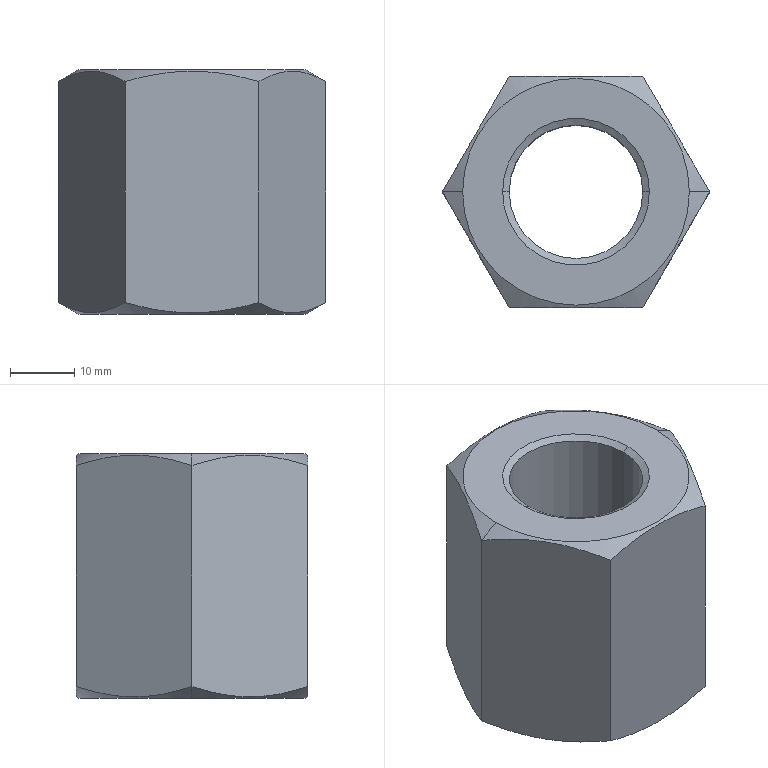Part | SolidWorks | features RevCut 2, Chamfer 1, Extrusion 1, LPattern 1 | 1 solid | 18 faces | box 41.569 x 36 x 38 mm | volume 29600 mm3 | cone 8 | plane 8 | cylinder 2 | commonest cylinder face diameters 20.752 x2
STEP:
#1=CARTESIAN_POINT('',(10.376,0.,-36.962));
#2=VERTEX_POINT('',#1);
#3=CARTESIAN_POINT('',(-10.376,0.,-36.962));
#4=VERTEX_POINT('',#3);
#5=CARTESIAN_POINT('',(0.,0.,-36.962));
#6=DIRECTION('',(0.,0.,-1.));
#7=DIRECTION('',(1.,0.,0.));
#8=AXIS2_PLACEMENT_3D('',#5,#6,#7);
#9=CIRCLE('',#8,10.376);
#10=EDGE_CURVE('',#2,#4,#9,.T.);
#11=ORIENTED_EDGE('',*,*,#10,.F.);
#12=CARTESIAN_POINT('',(10.975,0.,-38.));
#13=VERTEX_POINT('',#12);
#14=CARTESIAN_POINT('',(10.975,0.,-38.));
#15=DIRECTION('',(0.5,0.,-0.866));
#16=VECTOR('',#15,1000.);
#17=LINE('',#14,#16);
#18=EDGE_CURVE('',#2,#13,#17,.T.);
#19=ORIENTED_EDGE('',*,*,#18,.T.);
#20=CARTESIAN_POINT('',(-10.975,0.,-38.));
#21=VERTEX_POINT('',#20);
#22=CARTESIAN_POINT('',(0.,0.,-38.));
#23=DIRECTION('',(0.,0.,1.));
#24=DIRECTION('',(1.,0.,0.));
#25=AXIS2_PLACEMENT_3D('',#22,#23,#24);
#26=CIRCLE('',#25,10.975);
#27=EDGE_CURVE('',#21,#13,#26,.T.);
#28=ORIENTED_EDGE('',*,*,#27,.F.);
#29=CARTESIAN_POINT('',(-10.975,0.,-38.));
#30=DIRECTION('',(-0.5,0.,-0.866));
#31=VECTOR('',#30,1000.);
#32=LINE('',#29,#31);
#33=EDGE_CURVE('',#4,#21,#32,.T.);
#34=ORIENTED_EDGE('',*,*,#33,.F.);
#35=EDGE_LOOP('',(#11,#19,#28,#34));
#36=FACE_OUTER_BOUND('',#35,.T.);
#37=CARTESIAN_POINT('',(0.,0.,-38.));
#38=DIRECTION('',(0.,0.,-1.));
#39=DIRECTION('',(-1.,0.,0.));
#40=AXIS2_PLACEMENT_3D('',#37,#38,#39);
#41=CONICAL_SURFACE('',#40,10.975,0.5236);
#42=ADVANCED_FACE('',(#36),#41,.F.);
#43=CARTESIAN_POINT('',(-10.376,0.,-0.5991));
#44=VERTEX_POINT('',#43);
#45=CARTESIAN_POINT('',(10.376,0.,-0.5991));
#46=VERTEX_POINT('',#45);
#47=CARTESIAN_POINT('',(0.,0.,-0.5991));
#48=DIRECTION('',(0.,0.,1.));
#49=DIRECTION('',(1.,0.,0.));
#50=AXIS2_PLACEMENT_3D('',#47,#48,#49);
#51=CIRCLE('',#50,10.376);
#52=EDGE_CURVE('',#44,#46,#51,.T.);
#53=ORIENTED_EDGE('',*,*,#52,.F.);
#54=CARTESIAN_POINT('',(-11.414,0.,0.));
#55=VERTEX_POINT('',#54);
#56=CARTESIAN_POINT('',(-10.376,0.,-0.5991));
#57=DIRECTION('',(-0.866,0.,0.5));
#58=VECTOR('',#57,1000.);
#59=LINE('',#56,#58);
#60=EDGE_CURVE('',#44,#55,#59,.T.);
#61=ORIENTED_EDGE('',*,*,#60,.T.);
#62=CARTESIAN_POINT('',(11.414,0.,0.));
#63=VERTEX_POINT('',#62);
#64=CARTESIAN_POINT('',(0.,0.,0.));
#65=DIRECTION('',(0.,0.,-1.));
#66=DIRECTION('',(1.,0.,0.));
#67=AXIS2_PLACEMENT_3D('',#64,#65,#66);
#68=CIRCLE('',#67,11.414);
#69=EDGE_CURVE('',#63,#55,#68,.T.);
#70=ORIENTED_EDGE('',*,*,#69,.F.);
#71=CARTESIAN_POINT('',(10.376,0.,-0.5991));
#72=DIRECTION('',(0.866,0.,0.5));
#73=VECTOR('',#72,1000.);
#74=LINE('',#71,#73);
#75=EDGE_CURVE('',#46,#63,#74,.T.);
#76=ORIENTED_EDGE('',*,*,#75,.F.);
#77=EDGE_LOOP('',(#53,#61,#70,#76));
#78=FACE_OUTER_BOUND('',#77,.T.);
#79=CARTESIAN_POINT('',(0.,0.,-0.5991));
#80=DIRECTION('',(0.,0.,1.));
#81=DIRECTION('',(1.,0.,0.));
#82=AXIS2_PLACEMENT_3D('',#79,#80,#81);
#83=CONICAL_SURFACE('',#82,10.376,1.047);
#84=ADVANCED_FACE('',(#78),#83,.F.);
#85=CARTESIAN_POINT('',(-17.625,0.,0.));
#86=VERTEX_POINT('',#85);
#87=CARTESIAN_POINT('',(17.625,0.,0.));
#88=VERTEX_POINT('',#87);
#89=CARTESIAN_POINT('',(0.,0.,0.));
#90=DIRECTION('',(0.,0.,-1.));
#91=DIRECTION('',(-1.,0.,0.));
#92=AXIS2_PLACEMENT_3D('',#89,#90,#91);
#93=CIRCLE('',#92,17.625);
#94=EDGE_CURVE('',#86,#88,#93,.T.);
#95=ORIENTED_EDGE('',*,*,#94,.T.);
#96=CARTESIAN_POINT('',(20.785,0.,-1.824));
#97=VERTEX_POINT('',#96);
#98=CARTESIAN_POINT('',(17.625,0.,0.));
#99=DIRECTION('',(0.866,0.,-0.5));
#100=VECTOR('',#99,1000.);
#101=LINE('',#98,#100);
#102=EDGE_CURVE('',#88,#97,#101,.T.);
#103=ORIENTED_EDGE('',*,*,#102,.T.);
#104=CARTESIAN_POINT('',(10.392,18.,-1.824));
#105=VERTEX_POINT('',#104);
#106=CARTESIAN_POINT('',(20.785,0.,-1.824));
#107=CARTESIAN_POINT('',(19.936,1.47,-1.334));
#108=CARTESIAN_POINT('',(19.082,2.95,-0.9306));
#109=CARTESIAN_POINT('',(17.354,5.941,-0.3714));
#110=CARTESIAN_POINT('',(16.482,7.452,-0.2176));
#111=CARTESIAN_POINT('',(15.378,9.365,-0.2162));
#112=CARTESIAN_POINT('',(15.156,9.75,-0.2254));
#113=CARTESIAN_POINT('',(14.714,10.515,-0.2624));
#114=CARTESIAN_POINT('',(14.493,10.897,-0.2902));
#115=CARTESIAN_POINT('',(13.835,12.037,-0.4001));
#116=CARTESIAN_POINT('',(13.399,12.793,-0.5089));
#117=CARTESIAN_POINT('',(12.098,15.045,-0.929));
#118=CARTESIAN_POINT('',(11.242,16.529,-1.334));
#119=CARTESIAN_POINT('',(10.392,18.,-1.824));
#120=B_SPLINE_CURVE_WITH_KNOTS('',3,(#106,#107,#108,#109,#110,#111,#112,#113,#114,#115,#116,#117,#118,#119),.UNSPECIFIED.,.F.,.F.,(4,2,2,2,2,2,4),(0.000000238,0.005248,0.0105,0.01181,0.01312,0.01574,0.02099),.UNSPECIFIED.);
#121=EDGE_CURVE('',#97,#105,#120,.T.);
#122=ORIENTED_EDGE('',*,*,#121,.T.);
#123=CARTESIAN_POINT('',(-10.392,18.,-1.824));
#124=VERTEX_POINT('',#123);
#125=CARTESIAN_POINT('',(10.392,18.,-1.824));
#126=CARTESIAN_POINT('',(8.712,18.,-1.339));
#127=CARTESIAN_POINT('',(7.011,18.,-0.9354));
#128=CARTESIAN_POINT('',(4.408,18.,-0.5127));
#129=CARTESIAN_POINT('',(3.53,18.,-0.4024));
#130=CARTESIAN_POINT('',(1.762,18.,-0.254));
#131=CARTESIAN_POINT('',(0.8814,18.,-0.2166));
#132=CARTESIAN_POINT('',(-1.753,18.,-0.2163));
#133=CARTESIAN_POINT('',(-3.499,18.,-0.3672));
#134=CARTESIAN_POINT('',(-6.102,18.,-0.7869));
#135=CARTESIAN_POINT('',(-6.968,18.,-0.9587));
#136=CARTESIAN_POINT('',(-8.694,18.,-1.356));
#137=CARTESIAN_POINT('',(-9.547,18.,-1.58));
#138=CARTESIAN_POINT('',(-10.392,18.,-1.824));
#139=B_SPLINE_CURVE_WITH_KNOTS('',3,(#125,#126,#127,#128,#129,#130,#131,#132,#133,#134,#135,#136,#137,#138),.UNSPECIFIED.,.F.,.F.,(4,2,2,2,2,2,4),(0.007654,0.0129,0.01552,0.01814,0.02339,0.02601,0.02863),.UNSPECIFIED.);
#140=EDGE_CURVE('',#105,#124,#139,.T.);
#141=ORIENTED_EDGE('',*,*,#140,.T.);
#142=CARTESIAN_POINT('',(-20.785,0.,-1.824));
#143=VERTEX_POINT('',#142);
#144=CARTESIAN_POINT('',(-10.392,18.,-1.824));
#145=CARTESIAN_POINT('',(-11.241,16.53,-1.334));
#146=CARTESIAN_POINT('',(-12.095,15.05,-0.9306));
#147=CARTESIAN_POINT('',(-13.822,12.059,-0.3714));
#148=CARTESIAN_POINT('',(-14.695,10.548,-0.2176));
#149=CARTESIAN_POINT('',(-15.799,8.635,-0.2162));
#150=CARTESIAN_POINT('',(-16.021,8.25,-0.2254));
#151=CARTESIAN_POINT('',(-16.463,7.485,-0.2624));
#152=CARTESIAN_POINT('',(-16.684,7.103,-0.2902));
#153=CARTESIAN_POINT('',(-17.342,5.963,-0.4001));
#154=CARTESIAN_POINT('',(-17.778,5.207,-0.5089));
#155=CARTESIAN_POINT('',(-19.079,2.955,-0.929));
#156=CARTESIAN_POINT('',(-19.935,1.471,-1.334));
#157=CARTESIAN_POINT('',(-20.785,0.,-1.824));
#158=B_SPLINE_CURVE_WITH_KNOTS('',3,(#144,#145,#146,#147,#148,#149,#150,#151,#152,#153,#154,#155,#156,#157),.UNSPECIFIED.,.F.,.F.,(4,2,2,2,2,2,4),(0.000000238,0.005248,0.0105,0.01181,0.01312,0.01574,0.02099),.UNSPECIFIED.);
#159=EDGE_CURVE('',#124,#143,#158,.T.);
#160=ORIENTED_EDGE('',*,*,#159,.T.);
#161=CARTESIAN_POINT('',(-17.625,0.,0.));
#162=DIRECTION('',(-0.866,0.,-0.5));
#163=VECTOR('',#162,1000.);
#164=LINE('',#161,#163);
#165=EDGE_CURVE('',#86,#143,#164,.T.);
#166=ORIENTED_EDGE('',*,*,#165,.F.);
#167=EDGE_LOOP('',(#95,#103,#122,#141,#160,#166));
#168=FACE_OUTER_BOUND('',#167,.T.);
#169=CARTESIAN_POINT('',(0.,0.,0.));
#170=DIRECTION('',(0.,0.,-1.));
#171=DIRECTION('',(-1.,0.,0.));
#172=AXIS2_PLACEMENT_3D('',#169,#170,#171);
#173=CONICAL_SURFACE('',#172,17.625,1.047);
#174=ADVANCED_FACE('',(#168),#173,.T.);
#175=CARTESIAN_POINT('',(-17.625,0.,-38.));
#176=VERTEX_POINT('',#175);
#177=CARTESIAN_POINT('',(17.625,0.,-38.));
#178=VERTEX_POINT('',#177);
#179=CARTESIAN_POINT('',(0.,0.,-38.));
#180=DIRECTION('',(0.,0.,-1.));
#181=DIRECTION('',(-1.,0.,0.));
#182=AXIS2_PLACEMENT_3D('',#179,#180,#181);
#183=CIRCLE('',#182,17.625);
#184=EDGE_CURVE('',#176,#178,#183,.T.);
#185=ORIENTED_EDGE('',*,*,#184,.F.);
#186=CARTESIAN_POINT('',(-20.785,0.,-36.176));
#187=VERTEX_POINT('',#186);
#188=CARTESIAN_POINT('',(-20.785,0.,-36.176));
#189=DIRECTION('',(-0.866,0.,0.5));
#190=VECTOR('',#189,1000.);
#191=LINE('',#188,#190);
#192=EDGE_CURVE('',#176,#187,#191,.T.);
#193=ORIENTED_EDGE('',*,*,#192,.T.);
#194=CARTESIAN_POINT('',(-10.392,18.,-36.176));
#195=VERTEX_POINT('',#194);
#196=CARTESIAN_POINT('',(-20.785,0.,-36.176));
#197=CARTESIAN_POINT('',(-19.936,1.47,-36.666));
#198=CARTESIAN_POINT('',(-19.082,2.95,-37.069));
#199=CARTESIAN_POINT('',(-17.354,5.941,-37.629));
#200=CARTESIAN_POINT('',(-16.482,7.452,-37.782));
#201=CARTESIAN_POINT('',(-15.378,9.365,-37.784));
#202=CARTESIAN_POINT('',(-15.156,9.75,-37.775));
#203=CARTESIAN_POINT('',(-14.714,10.515,-37.738));
#204=CARTESIAN_POINT('',(-14.493,10.897,-37.71));
#205=CARTESIAN_POINT('',(-13.835,12.037,-37.6));
#206=CARTESIAN_POINT('',(-13.399,12.793,-37.491));
#207=CARTESIAN_POINT('',(-12.098,15.045,-37.071));
#208=CARTESIAN_POINT('',(-11.242,16.529,-36.666));
#209=CARTESIAN_POINT('',(-10.392,18.,-36.176));
#210=B_SPLINE_CURVE_WITH_KNOTS('',3,(#196,#197,#198,#199,#200,#201,#202,#203,#204,#205,#206,#207,#208,#209),.UNSPECIFIED.,.F.,.F.,(4,2,2,2,2,2,4),(0.000000238,0.005248,0.0105,0.01181,0.01312,0.01574,0.02099),.UNSPECIFIED.);
#211=EDGE_CURVE('',#187,#195,#210,.T.);
#212=ORIENTED_EDGE('',*,*,#211,.T.);
#213=CARTESIAN_POINT('',(10.392,18.,-36.176));
#214=VERTEX_POINT('',#213);
#215=CARTESIAN_POINT('',(-10.392,18.,-36.176));
#216=CARTESIAN_POINT('',(-9.547,18.,-36.42));
#217=CARTESIAN_POINT('',(-8.694,18.,-36.644));
#218=CARTESIAN_POINT('',(-6.968,18.,-37.041));
#219=CARTESIAN_POINT('',(-6.102,18.,-37.213));
#220=CARTESIAN_POINT('',(-3.499,18.,-37.633));
#221=CARTESIAN_POINT('',(-1.753,18.,-37.784));
#222=CARTESIAN_POINT('',(0.8814,18.,-37.783));
#223=CARTESIAN_POINT('',(1.762,18.,-37.746));
#224=CARTESIAN_POINT('',(3.53,18.,-37.598));
#225=CARTESIAN_POINT('',(4.408,18.,-37.487));
#226=CARTESIAN_POINT('',(7.011,18.,-37.065));
#227=CARTESIAN_POINT('',(8.712,18.,-36.661));
#228=CARTESIAN_POINT('',(10.392,18.,-36.176));
#229=B_SPLINE_CURVE_WITH_KNOTS('',3,(#215,#216,#217,#218,#219,#220,#221,#222,#223,#224,#225,#226,#227,#228),.UNSPECIFIED.,.F.,.F.,(4,2,2,2,2,2,4),(0.01851,0.02114,0.02377,0.02902,0.03165,0.03428,0.03954),.UNSPECIFIED.);
#230=EDGE_CURVE('',#195,#214,#229,.T.);
#231=ORIENTED_EDGE('',*,*,#230,.T.);
#232=CARTESIAN_POINT('',(20.785,0.,-36.176));
#233=VERTEX_POINT('',#232);
#234=CARTESIAN_POINT('',(10.392,18.,-36.176));
#235=CARTESIAN_POINT('',(11.241,16.53,-36.666));
#236=CARTESIAN_POINT('',(12.095,15.05,-37.069));
#237=CARTESIAN_POINT('',(13.822,12.059,-37.629));
#238=CARTESIAN_POINT('',(14.695,10.548,-37.782));
#239=CARTESIAN_POINT('',(15.799,8.635,-37.784));
#240=CARTESIAN_POINT('',(16.021,8.25,-37.775));
#241=CARTESIAN_POINT('',(16.463,7.485,-37.738));
#242=CARTESIAN_POINT('',(16.684,7.103,-37.71));
#243=CARTESIAN_POINT('',(17.342,5.963,-37.6));
#244=CARTESIAN_POINT('',(17.778,5.207,-37.491));
#245=CARTESIAN_POINT('',(19.079,2.955,-37.071));
#246=CARTESIAN_POINT('',(19.935,1.471,-36.666));
#247=CARTESIAN_POINT('',(20.785,0.,-36.176));
#248=B_SPLINE_CURVE_WITH_KNOTS('',3,(#234,#235,#236,#237,#238,#239,#240,#241,#242,#243,#244,#245,#246,#247),.UNSPECIFIED.,.F.,.F.,(4,2,2,2,2,2,4),(0.000000238,0.005248,0.0105,0.01181,0.01312,0.01574,0.02099),.UNSPECIFIED.);
#249=EDGE_CURVE('',#214,#233,#248,.T.);
#250=ORIENTED_EDGE('',*,*,#249,.T.);
#251=CARTESIAN_POINT('',(20.785,0.,-36.176));
#252=DIRECTION('',(0.866,0.,0.5));
#253=VECTOR('',#252,1000.);
#254=LINE('',#251,#253);
#255=EDGE_CURVE('',#178,#233,#254,.T.);
#256=ORIENTED_EDGE('',*,*,#255,.F.);
#257=EDGE_LOOP('',(#185,#193,#212,#231,#250,#256));
#258=FACE_OUTER_BOUND('',#257,.T.);
#259=CARTESIAN_POINT('',(0.,0.,-36.176));
#260=DIRECTION('',(0.,0.,1.));
#261=DIRECTION('',(1.,0.,0.));
#262=AXIS2_PLACEMENT_3D('',#259,#260,#261);
#263=CONICAL_SURFACE('',#262,20.785,1.047);
#264=ADVANCED_FACE('',(#258),#263,.T.);
#265=ORIENTED_EDGE('',*,*,#10,.T.);
#266=CARTESIAN_POINT('',(-10.376,0.,-38.));
#267=DIRECTION('',(0.,0.,1.));
#268=VECTOR('',#267,1000.);
#269=LINE('',#266,#268);
#270=EDGE_CURVE('',#4,#44,#269,.T.);
#271=ORIENTED_EDGE('',*,*,#270,.T.);
#272=ORIENTED_EDGE('',*,*,#52,.T.);
#273=CARTESIAN_POINT('',(10.376,0.,-38.));
#274=DIRECTION('',(0.,0.,1.));
#275=VECTOR('',#274,1000.);
#276=LINE('',#273,#275);
#277=EDGE_CURVE('',#2,#46,#276,.T.);
#278=ORIENTED_EDGE('',*,*,#277,.F.);
#279=EDGE_LOOP('',(#265,#271,#272,#278));
#280=FACE_OUTER_BOUND('',#279,.T.);
#281=CARTESIAN_POINT('',(0.,0.,-38.));
#282=DIRECTION('',(0.,0.,1.));
#283=DIRECTION('',(1.,0.,0.));
#284=AXIS2_PLACEMENT_3D('',#281,#282,#283);
#285=CYLINDRICAL_SURFACE('',#284,10.376);
#286=ADVANCED_FACE('',(#280),#285,.F.);
#287=CARTESIAN_POINT('',(-10.392,-18.,-1.824));
#288=VERTEX_POINT('',#287);
#289=CARTESIAN_POINT('',(10.392,-18.,-1.824));
#290=VERTEX_POINT('',#289);
#291=CARTESIAN_POINT('',(-10.392,-18.,-1.824));
#292=CARTESIAN_POINT('',(-9.547,-18.,-1.58));
#293=CARTESIAN_POINT('',(-8.694,-18.,-1.356));
#294=CARTESIAN_POINT('',(-6.968,-18.,-0.9587));
#295=CARTESIAN_POINT('',(-6.102,-18.,-0.7869));
#296=CARTESIAN_POINT('',(-3.499,-18.,-0.3672));
#297=CARTESIAN_POINT('',(-1.753,-18.,-0.2163));
#298=CARTESIAN_POINT('',(0.8814,-18.,-0.2166));
#299=CARTESIAN_POINT('',(1.762,-18.,-0.254));
#300=CARTESIAN_POINT('',(3.53,-18.,-0.4024));
#301=CARTESIAN_POINT('',(4.408,-18.,-0.5127));
#302=CARTESIAN_POINT('',(7.011,-18.,-0.9354));
#303=CARTESIAN_POINT('',(8.712,-18.,-1.339));
#304=CARTESIAN_POINT('',(10.392,-18.,-1.824));
#305=B_SPLINE_CURVE_WITH_KNOTS('',3,(#291,#292,#293,#294,#295,#296,#297,#298,#299,#300,#301,#302,#303,#304),.UNSPECIFIED.,.F.,.F.,(4,2,2,2,2,2,4),(0.01851,0.02114,0.02377,0.02902,0.03165,0.03428,0.03954),.UNSPECIFIED.);
#306=EDGE_CURVE('',#288,#290,#305,.T.);
#307=ORIENTED_EDGE('',*,*,#306,.F.);
#308=CARTESIAN_POINT('',(-10.392,-18.,-36.176));
#309=VERTEX_POINT('',#308);
#310=CARTESIAN_POINT('',(-10.392,-18.,-38.));
#311=DIRECTION('',(0.,0.,1.));
#312=VECTOR('',#311,1000.);
#313=LINE('',#310,#312);
#314=EDGE_CURVE('',#309,#288,#313,.T.);
#315=ORIENTED_EDGE('',*,*,#314,.F.);
#316=CARTESIAN_POINT('',(10.392,-18.,-36.176));
#317=VERTEX_POINT('',#316);
#318=CARTESIAN_POINT('',(10.392,-18.,-36.176));
#319=CARTESIAN_POINT('',(8.712,-18.,-36.661));
#320=CARTESIAN_POINT('',(7.011,-18.,-37.065));
#321=CARTESIAN_POINT('',(4.408,-18.,-37.487));
#322=CARTESIAN_POINT('',(3.53,-18.,-37.598));
#323=CARTESIAN_POINT('',(1.762,-18.,-37.746));
#324=CARTESIAN_POINT('',(0.8814,-18.,-37.783));
#325=CARTESIAN_POINT('',(-1.753,-18.,-37.784));
#326=CARTESIAN_POINT('',(-3.499,-18.,-37.633));
#327=CARTESIAN_POINT('',(-6.102,-18.,-37.213));
#328=CARTESIAN_POINT('',(-6.968,-18.,-37.041));
#329=CARTESIAN_POINT('',(-8.694,-18.,-36.644));
#330=CARTESIAN_POINT('',(-9.547,-18.,-36.42));
#331=CARTESIAN_POINT('',(-10.392,-18.,-36.176));
#332=B_SPLINE_CURVE_WITH_KNOTS('',3,(#318,#319,#320,#321,#322,#323,#324,#325,#326,#327,#328,#329,#330,#331),.UNSPECIFIED.,.F.,.F.,(4,2,2,2,2,2,4),(0.007654,0.0129,0.01552,0.01814,0.02339,0.02601,0.02863),.UNSPECIFIED.);
#333=EDGE_CURVE('',#317,#309,#332,.T.);
#334=ORIENTED_EDGE('',*,*,#333,.F.);
#335=CARTESIAN_POINT('',(10.392,-18.,-38.));
#336=DIRECTION('',(0.,0.,1.));
#337=VECTOR('',#336,1000.);
#338=LINE('',#335,#337);
#339=EDGE_CURVE('',#317,#290,#338,.T.);
#340=ORIENTED_EDGE('',*,*,#339,.T.);
#341=EDGE_LOOP('',(#307,#315,#334,#340));
#342=FACE_OUTER_BOUND('',#341,.T.);
#343=CARTESIAN_POINT('',(-10.392,-18.,-38.));
#344=DIRECTION('',(0.,-1.,0.));
#345=DIRECTION('',(0.,0.,-1.));
#346=AXIS2_PLACEMENT_3D('',#343,#344,#345);
#347=PLANE('',#346);
#348=ADVANCED_FACE('',(#342),#347,.T.);
#349=CARTESIAN_POINT('',(-20.785,0.,-1.824));
#350=CARTESIAN_POINT('',(-19.936,-1.47,-1.334));
#351=CARTESIAN_POINT('',(-19.082,-2.95,-0.9306));
#352=CARTESIAN_POINT('',(-17.354,-5.941,-0.3714));
#353=CARTESIAN_POINT('',(-16.482,-7.452,-0.2176));
#354=CARTESIAN_POINT('',(-15.378,-9.365,-0.2162));
#355=CARTESIAN_POINT('',(-15.156,-9.75,-0.2254));
#356=CARTESIAN_POINT('',(-14.714,-10.515,-0.2624));
#357=CARTESIAN_POINT('',(-14.493,-10.897,-0.2902));
#358=CARTESIAN_POINT('',(-13.835,-12.037,-0.4001));
#359=CARTESIAN_POINT('',(-13.399,-12.793,-0.5089));
#360=CARTESIAN_POINT('',(-12.098,-15.045,-0.929));
#361=CARTESIAN_POINT('',(-11.242,-16.529,-1.334));
#362=CARTESIAN_POINT('',(-10.392,-18.,-1.824));
#363=B_SPLINE_CURVE_WITH_KNOTS('',3,(#349,#350,#351,#352,#353,#354,#355,#356,#357,#358,#359,#360,#361,#362),.UNSPECIFIED.,.F.,.F.,(4,2,2,2,2,2,4),(0.000000238,0.005248,0.0105,0.01181,0.01312,0.01574,0.02099),.UNSPECIFIED.);
#364=EDGE_CURVE('',#143,#288,#363,.T.);
#365=ORIENTED_EDGE('',*,*,#364,.F.);
#366=CARTESIAN_POINT('',(-20.785,0.,-38.));
#367=DIRECTION('',(0.,0.,1.));
#368=VECTOR('',#367,1000.);
#369=LINE('',#366,#368);
#370=EDGE_CURVE('',#187,#143,#369,.T.);
#371=ORIENTED_EDGE('',*,*,#370,.F.);
#372=CARTESIAN_POINT('',(-10.392,-18.,-36.176));
#373=CARTESIAN_POINT('',(-11.241,-16.53,-36.666));
#374=CARTESIAN_POINT('',(-12.095,-15.05,-37.069));
#375=CARTESIAN_POINT('',(-13.822,-12.059,-37.629));
#376=CARTESIAN_POINT('',(-14.695,-10.548,-37.782));
#377=CARTESIAN_POINT('',(-15.799,-8.635,-37.784));
#378=CARTESIAN_POINT('',(-16.021,-8.25,-37.775));
#379=CARTESIAN_POINT('',(-16.463,-7.485,-37.738));
#380=CARTESIAN_POINT('',(-16.684,-7.103,-37.71));
#381=CARTESIAN_POINT('',(-17.342,-5.963,-37.6));
#382=CARTESIAN_POINT('',(-17.778,-5.207,-37.491));
#383=CARTESIAN_POINT('',(-19.079,-2.955,-37.071));
#384=CARTESIAN_POINT('',(-19.935,-1.471,-36.666));
#385=CARTESIAN_POINT('',(-20.785,0.,-36.176));
#386=B_SPLINE_CURVE_WITH_KNOTS('',3,(#372,#373,#374,#375,#376,#377,#378,#379,#380,#381,#382,#383,#384,#385),.UNSPECIFIED.,.F.,.F.,(4,2,2,2,2,2,4),(0.000000238,0.005248,0.0105,0.01181,0.01312,0.01574,0.02099),.UNSPECIFIED.);
#387=EDGE_CURVE('',#309,#187,#386,.T.);
#388=ORIENTED_EDGE('',*,*,#387,.F.);
#389=ORIENTED_EDGE('',*,*,#314,.T.);
#390=EDGE_LOOP('',(#365,#371,#388,#389));
#391=FACE_OUTER_BOUND('',#390,.T.);
#392=CARTESIAN_POINT('',(-20.785,0.,-38.));
#393=DIRECTION('',(-0.866,-0.5,0.));
#394=DIRECTION('',(0.5,-0.866,0.));
#395=AXIS2_PLACEMENT_3D('',#392,#393,#394);
#396=PLANE('',#395);
#397=ADVANCED_FACE('',(#391),#396,.T.);
#398=ORIENTED_EDGE('',*,*,#159,.F.);
#399=CARTESIAN_POINT('',(-10.392,18.,-38.));
#400=DIRECTION('',(0.,0.,1.));
#401=VECTOR('',#400,1000.);
#402=LINE('',#399,#401);
#403=EDGE_CURVE('',#195,#124,#402,.T.);
#404=ORIENTED_EDGE('',*,*,#403,.F.);
#405=ORIENTED_EDGE('',*,*,#211,.F.);
#406=ORIENTED_EDGE('',*,*,#370,.T.);
#407=EDGE_LOOP('',(#398,#404,#405,#406));
#408=FACE_OUTER_BOUND('',#407,.T.);
#409=CARTESIAN_POINT('',(-10.392,18.,-38.));
#410=DIRECTION('',(-0.866,0.5,0.));
#411=DIRECTION('',(-0.5,-0.866,0.));
#412=AXIS2_PLACEMENT_3D('',#409,#410,#411);
#413=PLANE('',#412);
#414=ADVANCED_FACE('',(#408),#413,.T.);
#415=ORIENTED_EDGE('',*,*,#140,.F.);
#416=CARTESIAN_POINT('',(10.392,18.,-38.));
#417=DIRECTION('',(0.,0.,1.));
#418=VECTOR('',#417,1000.);
#419=LINE('',#416,#418);
#420=EDGE_CURVE('',#214,#105,#419,.T.);
#421=ORIENTED_EDGE('',*,*,#420,.F.);
#422=ORIENTED_EDGE('',*,*,#230,.F.);
#423=ORIENTED_EDGE('',*,*,#403,.T.);
#424=EDGE_LOOP('',(#415,#421,#422,#423));
#425=FACE_OUTER_BOUND('',#424,.T.);
#426=CARTESIAN_POINT('',(10.392,18.,-38.));
#427=DIRECTION('',(0.,1.,0.));
#428=DIRECTION('',(-1.,0.,0.));
#429=AXIS2_PLACEMENT_3D('',#426,#427,#428);
#430=PLANE('',#429);
#431=ADVANCED_FACE('',(#425),#430,.T.);
#432=ORIENTED_EDGE('',*,*,#121,.F.);
#433=CARTESIAN_POINT('',(20.785,0.,-38.));
#434=DIRECTION('',(0.,0.,1.));
#435=VECTOR('',#434,1000.);
#436=LINE('',#433,#435);
#437=EDGE_CURVE('',#233,#97,#436,.T.);
#438=ORIENTED_EDGE('',*,*,#437,.F.);
#439=ORIENTED_EDGE('',*,*,#249,.F.);
#440=ORIENTED_EDGE('',*,*,#420,.T.);
#441=EDGE_LOOP('',(#432,#438,#439,#440));
#442=FACE_OUTER_BOUND('',#441,.T.);
#443=CARTESIAN_POINT('',(20.785,0.,-38.));
#444=DIRECTION('',(0.866,0.5,0.));
#445=DIRECTION('',(-0.5,0.866,0.));
#446=AXIS2_PLACEMENT_3D('',#443,#444,#445);
#447=PLANE('',#446);
#448=ADVANCED_FACE('',(#442),#447,.T.);
#449=CARTESIAN_POINT('',(10.392,-18.,-1.824));
#450=CARTESIAN_POINT('',(11.241,-16.53,-1.334));
#451=CARTESIAN_POINT('',(12.095,-15.05,-0.9306));
#452=CARTESIAN_POINT('',(13.822,-12.059,-0.3714));
#453=CARTESIAN_POINT('',(14.695,-10.548,-0.2176));
#454=CARTESIAN_POINT('',(15.799,-8.635,-0.2162));
#455=CARTESIAN_POINT('',(16.021,-8.25,-0.2254));
#456=CARTESIAN_POINT('',(16.463,-7.485,-0.2624));
#457=CARTESIAN_POINT('',(16.684,-7.103,-0.2902));
#458=CARTESIAN_POINT('',(17.342,-5.963,-0.4001));
#459=CARTESIAN_POINT('',(17.778,-5.207,-0.5089));
#460=CARTESIAN_POINT('',(19.079,-2.955,-0.929));
#461=CARTESIAN_POINT('',(19.935,-1.471,-1.334));
#462=CARTESIAN_POINT('',(20.785,0.,-1.824));
#463=B_SPLINE_CURVE_WITH_KNOTS('',3,(#449,#450,#451,#452,#453,#454,#455,#456,#457,#458,#459,#460,#461,#462),.UNSPECIFIED.,.F.,.F.,(4,2,2,2,2,2,4),(0.000000238,0.005248,0.0105,0.01181,0.01312,0.01574,0.02099),.UNSPECIFIED.);
#464=EDGE_CURVE('',#290,#97,#463,.T.);
#465=ORIENTED_EDGE('',*,*,#464,.F.);
#466=ORIENTED_EDGE('',*,*,#339,.F.);
#467=CARTESIAN_POINT('',(20.785,0.,-36.176));
#468=CARTESIAN_POINT('',(19.936,-1.47,-36.666));
#469=CARTESIAN_POINT('',(19.082,-2.95,-37.069));
#470=CARTESIAN_POINT('',(17.354,-5.941,-37.629));
#471=CARTESIAN_POINT('',(16.482,-7.452,-37.782));
#472=CARTESIAN_POINT('',(15.378,-9.365,-37.784));
#473=CARTESIAN_POINT('',(15.156,-9.75,-37.775));
#474=CARTESIAN_POINT('',(14.714,-10.515,-37.738));
#475=CARTESIAN_POINT('',(14.493,-10.897,-37.71));
#476=CARTESIAN_POINT('',(13.835,-12.037,-37.6));
#477=CARTESIAN_POINT('',(13.399,-12.793,-37.491));
#478=CARTESIAN_POINT('',(12.098,-15.045,-37.071));
#479=CARTESIAN_POINT('',(11.242,-16.529,-36.666));
#480=CARTESIAN_POINT('',(10.392,-18.,-36.176));
#481=B_SPLINE_CURVE_WITH_KNOTS('',3,(#467,#468,#469,#470,#471,#472,#473,#474,#475,#476,#477,#478,#479,#480),.UNSPECIFIED.,.F.,.F.,(4,2,2,2,2,2,4),(0.000000238,0.005248,0.0105,0.01181,0.01312,0.01574,0.02099),.UNSPECIFIED.);
#482=EDGE_CURVE('',#233,#317,#481,.T.);
#483=ORIENTED_EDGE('',*,*,#482,.F.);
#484=ORIENTED_EDGE('',*,*,#437,.T.);
#485=EDGE_LOOP('',(#465,#466,#483,#484));
#486=FACE_OUTER_BOUND('',#485,.T.);
#487=CARTESIAN_POINT('',(10.392,-18.,-38.));
#488=DIRECTION('',(0.866,-0.5,0.));
#489=DIRECTION('',(0.5,0.866,0.));
#490=AXIS2_PLACEMENT_3D('',#487,#488,#489);
#491=PLANE('',#490);
#492=ADVANCED_FACE('',(#486),#491,.T.);
#493=ORIENTED_EDGE('',*,*,#27,.T.);
#494=CARTESIAN_POINT('',(0.,0.,-38.));
#495=DIRECTION('',(0.,0.,1.));
#496=DIRECTION('',(1.,0.,0.));
#497=AXIS2_PLACEMENT_3D('',#494,#495,#496);
#498=CIRCLE('',#497,10.975);
#499=EDGE_CURVE('',#13,#21,#498,.T.);
#500=ORIENTED_EDGE('',*,*,#499,.T.);
#501=EDGE_LOOP('',(#493,#500));
#502=FACE_BOUND('',#501,.T.);
#503=CARTESIAN_POINT('',(0.,0.,-38.));
#504=DIRECTION('',(0.,0.,-1.));
#505=DIRECTION('',(-1.,0.,0.));
#506=AXIS2_PLACEMENT_3D('',#503,#504,#505);
#507=CIRCLE('',#506,17.625);
#508=EDGE_CURVE('',#178,#176,#507,.T.);
#509=ORIENTED_EDGE('',*,*,#508,.T.);
#510=ORIENTED_EDGE('',*,*,#184,.T.);
#511=EDGE_LOOP('',(#509,#510));
#512=FACE_OUTER_BOUND('',#511,.T.);
#513=CARTESIAN_POINT('',(10.392,-18.,-38.));
#514=DIRECTION('',(0.,0.,1.));
#515=DIRECTION('',(1.,0.,0.));
#516=AXIS2_PLACEMENT_3D('',#513,#514,#515);
#517=PLANE('',#516);
#518=ADVANCED_FACE('',(#502,#512),#517,.F.);
#519=ORIENTED_EDGE('',*,*,#69,.T.);
#520=CARTESIAN_POINT('',(0.,0.,0.));
#521=DIRECTION('',(0.,0.,-1.));
#522=DIRECTION('',(1.,0.,0.));
#523=AXIS2_PLACEMENT_3D('',#520,#521,#522);
#524=CIRCLE('',#523,11.414);
#525=EDGE_CURVE('',#55,#63,#524,.T.);
#526=ORIENTED_EDGE('',*,*,#525,.T.);
#527=EDGE_LOOP('',(#519,#526));
#528=FACE_BOUND('',#527,.T.);
#529=ORIENTED_EDGE('',*,*,#94,.F.);
#530=CARTESIAN_POINT('',(0.,0.,0.));
#531=DIRECTION('',(0.,0.,-1.));
#532=DIRECTION('',(-1.,0.,0.));
#533=AXIS2_PLACEMENT_3D('',#530,#531,#532);
#534=CIRCLE('',#533,17.625);
#535=EDGE_CURVE('',#88,#86,#534,.T.);
#536=ORIENTED_EDGE('',*,*,#535,.F.);
#537=EDGE_LOOP('',(#529,#536));
#538=FACE_OUTER_BOUND('',#537,.T.);
#539=CARTESIAN_POINT('',(10.392,-18.,0.));
#540=DIRECTION('',(0.,0.,1.));
#541=DIRECTION('',(1.,0.,0.));
#542=AXIS2_PLACEMENT_3D('',#539,#540,#541);
#543=PLANE('',#542);
#544=ADVANCED_FACE('',(#528,#538),#543,.T.);
#545=ORIENTED_EDGE('',*,*,#270,.F.);
#546=CARTESIAN_POINT('',(0.,0.,-36.962));
#547=DIRECTION('',(0.,0.,-1.));
#548=DIRECTION('',(1.,0.,0.));
#549=AXIS2_PLACEMENT_3D('',#546,#547,#548);
#550=CIRCLE('',#549,10.376);
#551=EDGE_CURVE('',#4,#2,#550,.T.);
#552=ORIENTED_EDGE('',*,*,#551,.T.);
#553=ORIENTED_EDGE('',*,*,#277,.T.);
#554=CARTESIAN_POINT('',(0.,0.,-0.5991));
#555=DIRECTION('',(0.,0.,1.));
#556=DIRECTION('',(1.,0.,0.));
#557=AXIS2_PLACEMENT_3D('',#554,#555,#556);
#558=CIRCLE('',#557,10.376);
#559=EDGE_CURVE('',#46,#44,#558,.T.);
#560=ORIENTED_EDGE('',*,*,#559,.T.);
#561=EDGE_LOOP('',(#545,#552,#553,#560));
#562=FACE_OUTER_BOUND('',#561,.T.);
#563=CARTESIAN_POINT('',(0.,0.,-38.));
#564=DIRECTION('',(0.,0.,1.));
#565=DIRECTION('',(1.,0.,0.));
#566=AXIS2_PLACEMENT_3D('',#563,#564,#565);
#567=CYLINDRICAL_SURFACE('',#566,10.376);
#568=ADVANCED_FACE('',(#562),#567,.F.);
#569=ORIENTED_EDGE('',*,*,#192,.F.);
#570=ORIENTED_EDGE('',*,*,#508,.F.);
#571=ORIENTED_EDGE('',*,*,#255,.T.);
#572=ORIENTED_EDGE('',*,*,#482,.T.);
#573=ORIENTED_EDGE('',*,*,#333,.T.);
#574=ORIENTED_EDGE('',*,*,#387,.T.);
#575=EDGE_LOOP('',(#569,#570,#571,#572,#573,#574));
#576=FACE_OUTER_BOUND('',#575,.T.);
#577=CARTESIAN_POINT('',(0.,0.,-36.176));
#578=DIRECTION('',(0.,0.,1.));
#579=DIRECTION('',(1.,0.,0.));
#580=AXIS2_PLACEMENT_3D('',#577,#578,#579);
#581=CONICAL_SURFACE('',#580,20.785,1.047);
#582=ADVANCED_FACE('',(#576),#581,.T.);
#583=ORIENTED_EDGE('',*,*,#102,.F.);
#584=ORIENTED_EDGE('',*,*,#535,.T.);
#585=ORIENTED_EDGE('',*,*,#165,.T.);
#586=ORIENTED_EDGE('',*,*,#364,.T.);
#587=ORIENTED_EDGE('',*,*,#306,.T.);
#588=ORIENTED_EDGE('',*,*,#464,.T.);
#589=EDGE_LOOP('',(#583,#584,#585,#586,#587,#588));
#590=FACE_OUTER_BOUND('',#589,.T.);
#591=CARTESIAN_POINT('',(0.,0.,0.));
#592=DIRECTION('',(0.,0.,-1.));
#593=DIRECTION('',(-1.,0.,0.));
#594=AXIS2_PLACEMENT_3D('',#591,#592,#593);
#595=CONICAL_SURFACE('',#594,17.625,1.047);
#596=ADVANCED_FACE('',(#590),#595,.T.);
#597=ORIENTED_EDGE('',*,*,#60,.F.);
#598=ORIENTED_EDGE('',*,*,#559,.F.);
#599=ORIENTED_EDGE('',*,*,#75,.T.);
#600=ORIENTED_EDGE('',*,*,#525,.F.);
#601=EDGE_LOOP('',(#597,#598,#599,#600));
#602=FACE_OUTER_BOUND('',#601,.T.);
#603=CARTESIAN_POINT('',(0.,0.,-0.5991));
#604=DIRECTION('',(0.,0.,1.));
#605=DIRECTION('',(1.,0.,0.));
#606=AXIS2_PLACEMENT_3D('',#603,#604,#605);
#607=CONICAL_SURFACE('',#606,10.376,1.047);
#608=ADVANCED_FACE('',(#602),#607,.F.);
#609=ORIENTED_EDGE('',*,*,#18,.F.);
#610=ORIENTED_EDGE('',*,*,#551,.F.);
#611=ORIENTED_EDGE('',*,*,#33,.T.);
#612=ORIENTED_EDGE('',*,*,#499,.F.);
#613=EDGE_LOOP('',(#609,#610,#611,#612));
#614=FACE_OUTER_BOUND('',#613,.T.);
#615=CARTESIAN_POINT('',(0.,0.,-38.));
#616=DIRECTION('',(0.,0.,-1.));
#617=DIRECTION('',(-1.,0.,0.));
#618=AXIS2_PLACEMENT_3D('',#615,#616,#617);
#619=CONICAL_SURFACE('',#618,10.975,0.5236);
#620=ADVANCED_FACE('',(#614),#619,.F.);
#621=CLOSED_SHELL('',(#42,#84,#174,#264,#286,#348,#397,#414,#431,#448,#492,#518,#544,#568,#582,#596,#608,#620));
#622=MANIFOLD_SOLID_BREP('',#621);
#623=CARTESIAN_POINT('',(0.,0.,0.));
#624=DIRECTION('',(0.,0.,1.));
#625=DIRECTION('',(1.,0.,0.));
#626=AXIS2_PLACEMENT_3D('',#623,#624,#625);
#627=(LENGTH_UNIT()NAMED_UNIT(*)SI_UNIT(.MILLI.,.METRE.));
#628=UNCERTAINTY_MEASURE_WITH_UNIT(LENGTH_MEASURE(0.00001),#627,'','');
#629=(NAMED_UNIT(*)PLANE_ANGLE_UNIT()SI_UNIT($,.RADIAN.));
#630=(NAMED_UNIT(*)SI_UNIT($,.STERADIAN.)SOLID_ANGLE_UNIT());
#631=(GEOMETRIC_REPRESENTATION_CONTEXT(3)GLOBAL_UNCERTAINTY_ASSIGNED_CONTEXT((#628))GLOBAL_UNIT_ASSIGNED_CONTEXT((#627,#629,#630))REPRESENTATION_CONTEXT('',''));
#632=ADVANCED_BREP_SHAPE_REPRESENTATION('',(#622,#626),#631);